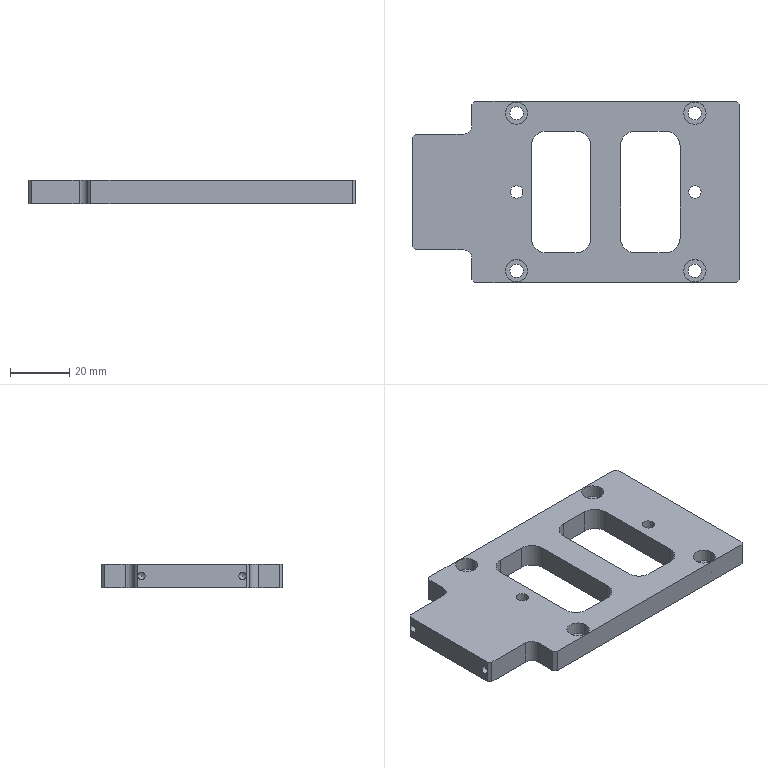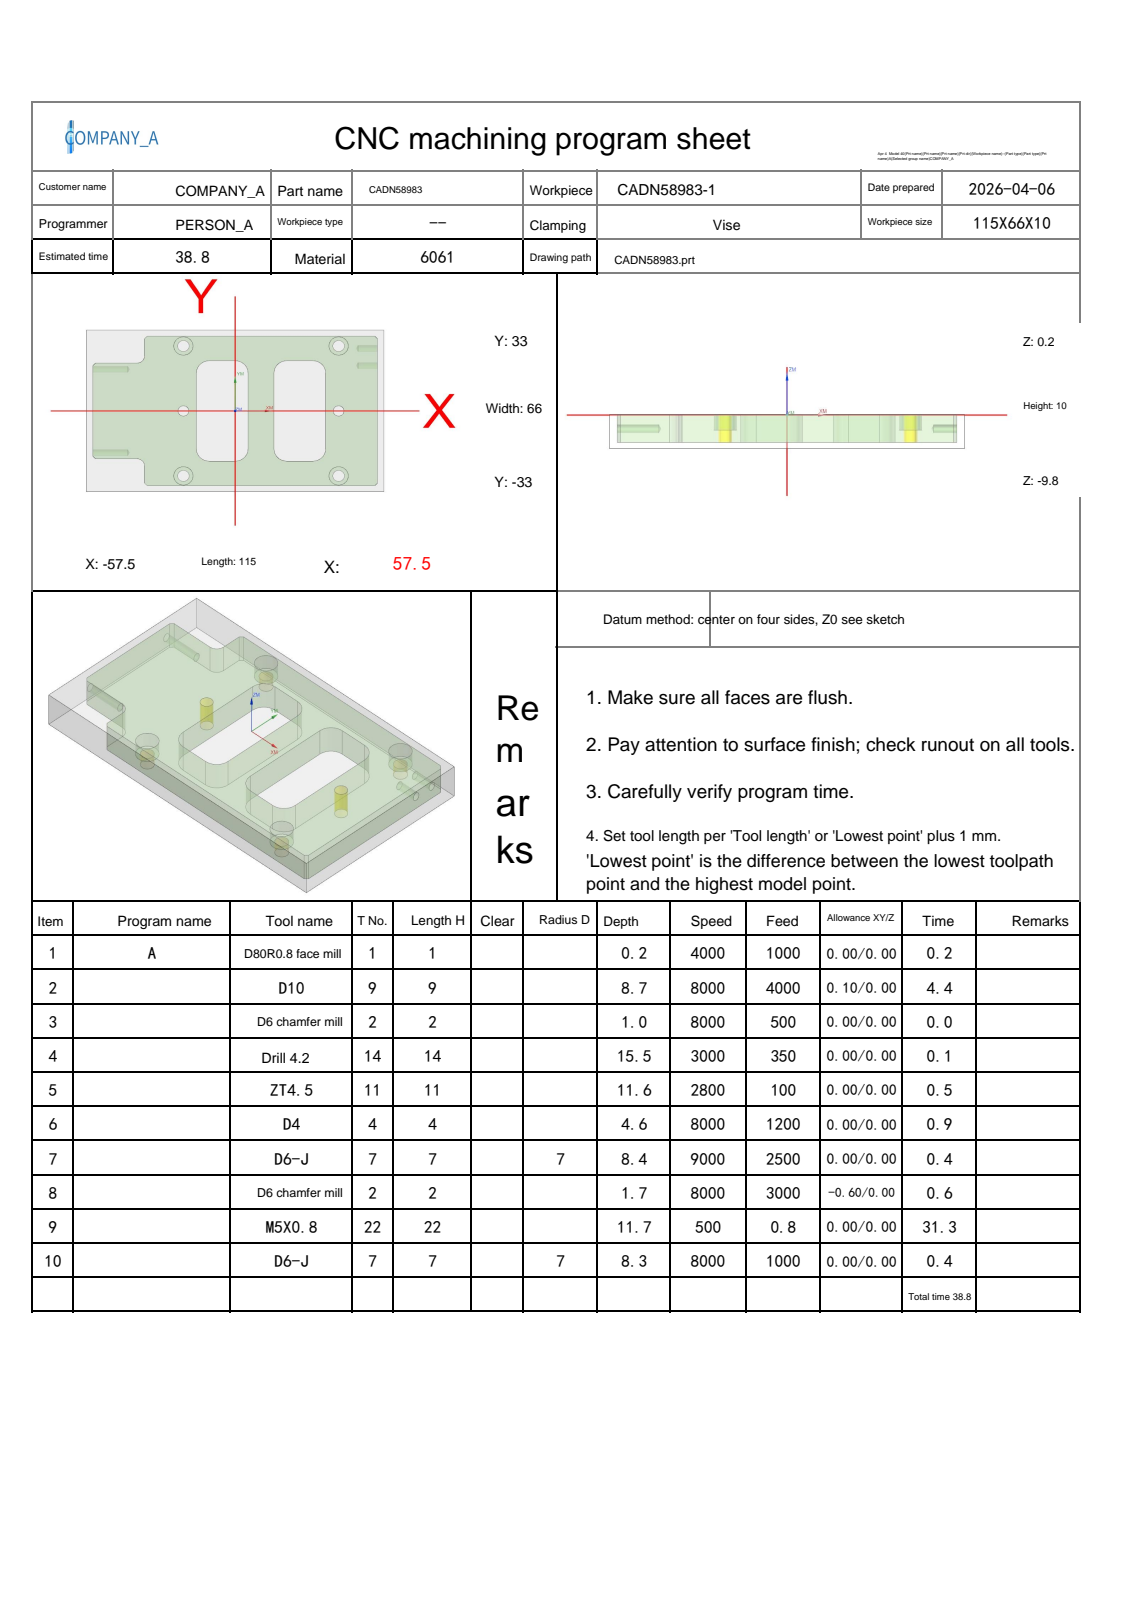NC program | NX | posted by the shop | part box 110 x 61 x 8 mm
Lines 4151 to 4510 of 4510:
N8 T02 M06
(D6 chamfer mill  D=6. R=0. H=02 ce=0.00 di=0.00)
G00 G90 G54 X9.75 Y32.628 M03 S8000
G43 H02 Z20.
M08
Z2.099
G01 Z-1.5 F3000.
G03 X9.67 Y32.328 I.52 J-.3
X9.97 Y31.808 I.6 J0.0
G01 X10. Y31.8
X54.
X54.254 Y31.775
X54.497 Y31.701
X54.722 Y31.581
X54.919 Y31.419
X55.919 Y30.419
X56.081 Y30.222
X56.201 Y29.997
X56.275 Y29.754
X56.3 Y29.5
Y-29.5
X56.275 Y-29.754
X56.201 Y-29.997
X56.081 Y-30.222
X55.919 Y-30.419
X54.919 Y-31.419
X54.722 Y-31.581
X54.497 Y-31.701
X54.254 Y-31.775
X54. Y-31.8
X-34.
X-34.254 Y-31.775
X-34.497 Y-31.701
X-34.722 Y-31.581
X-34.919 Y-31.419
X-35.919 Y-30.419
X-36.081 Y-30.222
X-36.201 Y-29.997
X-36.275 Y-29.754
X-36.3 Y-29.5
Y-22.5
G03 X-38. Y-20.8 I-1.7 J0.0
G01 X-54.
X-54.254 Y-20.775
X-54.497 Y-20.701
X-54.722 Y-20.581
X-54.919 Y-20.419
X-55.919 Y-19.419
X-56.081 Y-19.222
X-56.201 Y-18.997
X-56.275 Y-18.754
X-56.3 Y-18.5
Y18.5
X-56.275 Y18.754
X-56.201 Y18.997
X-56.081 Y19.222
X-55.919 Y19.419
X-54.919 Y20.419
X-54.722 Y20.581
X-54.497 Y20.701
X-54.254 Y20.775
X-54. Y20.8
X-38.
G03 X-36.3 Y22.5 I0.0 J1.7
G01 Y29.5
X-36.275 Y29.754
X-36.201 Y29.997
X-36.081 Y30.222
X-35.919 Y30.419
X-34.919 Y31.419
X-34.722 Y31.581
X-34.497 Y31.701
X-34.254 Y31.775
X-34. Y31.8
X10.
X10.03 Y31.808
G03 X10.33 Y32.328 I-.3 J.52
X10.25 Y32.628 I-.6 J0.0
G01 Z2.099
G00 Z20.
X2.872 Y-.25
Z2.099
G01 Z-1.5
G03 X3.172 Y-.33 I.3 J.52
X3.692 Y-.03 I0.0 J.6
G01 X3.7 Y0.0
Y15.5
G03 X0.0 Y19.2 I-3.7 J0.0
G01 X-10.
G03 X-13.7 Y15.5 I0.0 J-3.7
G01 Y-15.5
G03 X-10. Y-19.2 I3.7 J0.0
G01 X0.0
G03 X3.7 Y-15.5 I0.0 J3.7
G01 Y0.0
X3.692 Y.03
G03 X3.172 Y.33 I-.52 J-.3
X2.872 Y.25 I0.0 J-.6
G01 Z2.099
G00 Z20.
X17.128
Z2.099
G01 Z-1.5
G03 X16.828 Y.33 I-.3 J-.52
X16.308 Y.03 I0.0 J-.6
G01 X16.3 Y0.0
Y-15.5
G03 X20. Y-19.2 I3.7 J0.0
G01 X30.
G03 X33.7 Y-15.5 I0.0 J3.7
G01 Y15.5
G03 X30. Y19.2 I-3.7 J0.0
G01 X20.
G03 X16.3 Y15.5 I0.0 J-3.7
G01 Y0.0
X16.308 Y-.03
G03 X16.828 Y-.33 I.52 J.3
X17.128 Y-.25 I0.0 J.6
G01 Z2.099
G00 Z20.
G00 G90 X-19.907 Y-.694 M03 S8000
Z20.
Z-.5
G01 Z-1. F500.
X-19.8 Y-1.5
G03 X-18.3 Y0.0 I0.0 J1.5
X-20. Y1.7 I-1.7 J0.0
X-21.7 Y0.0 I0.0 J-1.7
X-20. Y-1.7 I1.7 J0.0
X-18.3 Y0.0 I0.0 J1.7
X-19.8 Y1.5 I-1.5 J0.0
G01 X-19.907 Y.694
Z-.5
G00 Z20.
X40.093 Y-.694
Z-.5
G01 Z-1.
X40.2 Y-1.5
G03 X41.7 Y0.0 I0.0 J1.5
X40. Y1.7 I-1.7 J0.0
X38.3 Y0.0 I0.0 J-1.7
X40. Y-1.7 I1.7 J0.0
X41.7 Y0.0 I0.0 J1.7
X40.2 Y1.5 I-1.5 J0.0
G01 X40.093 Y.694
Z-.5
G00 Z20.
G00 G90 X36.949 Y-26.469 M03 S8000
Z20.
Z2.5
G01 X36.947 Y-26.5 Z2.489 F500.
X36.971 Y-26.882 Z2.349
X37.042 Y-27.257 Z2.21
X37.16 Y-27.621 Z2.071
X37.323 Y-27.968 Z1.932
X37.527 Y-28.291 Z1.793
X37.771 Y-28.586 Z1.653
X38.049 Y-28.848 Z1.514
X38.358 Y-29.074 Z1.375
X38.592 Y-29.209 Z1.277
X38.942 Y-29.364 Z1.137
X39.308 Y-29.474 Z.998
X39.686 Y-29.537 Z.859
X40.068 Y-29.552 Z.72
X40.449 Y-29.52 Z.581
X40.823 Y-29.44 Z.441
X41.184 Y-29.314 Z.302
X41.527 Y-29.144 Z.163
X41.845 Y-28.932 Z.024
X42.135 Y-28.683 Z-.116
X42.391 Y-28.399 Z-.255
X42.609 Y-28.085 Z-.394
X42.787 Y-27.746 Z-.533
X42.921 Y-27.388 Z-.672
X43.009 Y-27.016 Z-.812
X43.05 Y-26.635 Z-.951
Y-26.5 Z-1.
G03 X40. Y-23.45 I-3.05 J0.0
X36.95 Y-26.5 I0.0 J-3.05
X40. Y-29.55 I3.05 J0.0
X43.05 Y-26.5 I0.0 J3.05
X43.009 Y-26.002 I-3.05 J0.0
G01 Z1.5
G00 Z20.
X36.949 Y26.531
Z2.5
G01 X36.947 Y26.5 Z2.489
X36.971 Y26.118 Z2.349
X37.042 Y25.743 Z2.21
X37.16 Y25.379 Z2.071
X37.323 Y25.032 Z1.932
X37.527 Y24.709 Z1.793
X37.771 Y24.414 Z1.653
X38.049 Y24.152 Z1.514
X38.358 Y23.926 Z1.375
X38.592 Y23.791 Z1.277
X38.942 Y23.636 Z1.137
X39.308 Y23.526 Z.998
X39.686 Y23.463 Z.859
X40.068 Y23.448 Z.72
X40.449 Y23.48 Z.581
X40.823 Y23.56 Z.441
X41.184 Y23.686 Z.302
X41.527 Y23.856 Z.163
X41.845 Y24.068 Z.024
X42.135 Y24.317 Z-.116
X42.391 Y24.601 Z-.255
X42.609 Y24.915 Z-.394
X42.787 Y25.254 Z-.533
X42.921 Y25.612 Z-.672
X43.009 Y25.984 Z-.812
X43.05 Y26.365 Z-.951
Y26.5 Z-1.
G03 X40. Y29.55 I-3.05 J0.0
X36.95 Y26.5 I0.0 J-3.05
X40. Y23.45 I3.05 J0.0
X43.05 Y26.5 I0.0 J3.05
X43.009 Y26.998 I-3.05 J0.0
G01 Z1.5
G00 Z20.
X-23.051 Y26.531
Z2.5
G01 X-23.053 Y26.5 Z2.489
X-23.029 Y26.118 Z2.349
X-22.958 Y25.743 Z2.21
X-22.84 Y25.379 Z2.071
X-22.677 Y25.032 Z1.932
X-22.473 Y24.709 Z1.793
X-22.229 Y24.414 Z1.653
X-21.951 Y24.152 Z1.514
X-21.642 Y23.926 Z1.375
X-21.408 Y23.791 Z1.277
X-21.058 Y23.636 Z1.137
X-20.692 Y23.526 Z.998
X-20.314 Y23.463 Z.859
X-19.932 Y23.448 Z.72
X-19.551 Y23.48 Z.581
X-19.177 Y23.56 Z.441
X-18.816 Y23.686 Z.302
X-18.474 Y23.856 Z.163
X-18.155 Y24.068 Z.024
X-17.865 Y24.317 Z-.116
X-17.609 Y24.601 Z-.255
X-17.391 Y24.915 Z-.394
X-17.213 Y25.254 Z-.533
X-17.079 Y25.612 Z-.672
X-16.991 Y25.984 Z-.812
X-16.95 Y26.365 Z-.951
Y26.5 Z-1.
G03 X-20. Y29.55 I-3.05 J0.0
X-23.05 Y26.5 I0.0 J-3.05
X-20. Y23.45 I3.05 J0.0
X-16.95 Y26.5 I0.0 J3.05
X-16.991 Y26.998 I-3.05 J0.0
G01 Z1.5
G00 Z20.
X-23.051 Y-26.469
Z2.5
G01 X-23.053 Y-26.5 Z2.489
X-23.029 Y-26.882 Z2.349
X-22.958 Y-27.257 Z2.21
X-22.84 Y-27.621 Z2.071
X-22.677 Y-27.968 Z1.932
X-22.473 Y-28.291 Z1.793
X-22.229 Y-28.586 Z1.653
X-21.951 Y-28.848 Z1.514
X-21.642 Y-29.074 Z1.375
X-21.408 Y-29.209 Z1.277
X-21.058 Y-29.364 Z1.137
X-20.692 Y-29.474 Z.998
X-20.314 Y-29.537 Z.859
X-19.932 Y-29.552 Z.72
X-19.551 Y-29.52 Z.581
X-19.177 Y-29.44 Z.441
X-18.816 Y-29.314 Z.302
X-18.474 Y-29.144 Z.163
X-18.155 Y-28.932 Z.024
X-17.865 Y-28.683 Z-.116
X-17.609 Y-28.399 Z-.255
X-17.391 Y-28.085 Z-.394
X-17.213 Y-27.746 Z-.533
X-17.079 Y-27.388 Z-.672
X-16.991 Y-27.016 Z-.812
X-16.95 Y-26.635 Z-.951
Y-26.5 Z-1.
G03 X-20. Y-23.45 I-3.05 J0.0
X-23.05 Y-26.5 I0.0 J-3.05
X-20. Y-29.55 I3.05 J0.0
X-16.95 Y-26.5 I0.0 J3.05
X-16.991 Y-26.002 I-3.05 J0.0
G01 Z1.5
G00 Z20.
G91 G28 Z0.0
M05
M09
G91 G28 Z0.0
M01
N9 T22 M06
(M5X0.8 D=4.2 DR_a=180 H=22)
G00 G90 G54 X-20. Y0.0 M03 S500
G43 H22 Z20.
M08
G95
G98 G84 X-20. Y0.0 Z-11.5 R1. F.8 Q3.
X40.
G80
G94
G00 Z20.
G91 G28 Z0.0
M05
M09
G91 G28 Z0.0
M01
N10 T07 M06
(D6-J  D=6. R=0. H=07 ce=0.00 di=0.00)
G00 G90 G54 X-35.017 Y34.573 M03 S8000
G43 H07 Z20.
M08
Z-7.6
G01 Z-8.1 F1000.
G41 D07
X-34.992 Y34.375
G03 X-34. Y33.5 I.992 J.125
G01 X54.
G02 X56.121 Y32.621 I0.0 J-3.
G01 X57.121 Y31.621
G02 X58. Y29.5 I-2.121 J-2.121
G01 Y-29.5
G02 X57.121 Y-31.621 I-3. J0.0
G01 X56.121 Y-32.621
G02 X54. Y-33.5 I-2.121 J2.121
G01 X-34.
G02 X-36.121 Y-32.621 I0.0 J3.
G01 X-37.121 Y-31.621
G02 X-38. Y-29.5 I2.121 J2.121
G01 Y-22.5
X-54.
G02 X-56.121 Y-21.621 I0.0 J3.
G01 X-57.121 Y-20.621
G02 X-58. Y-18.5 I2.121 J2.121
G01 Y18.5
G02 X-57.121 Y20.621 I3. J0.0
G01 X-56.121 Y21.621
G02 X-54. Y22.5 I2.121 J-2.121
G01 X-38.
Y29.5
G02 X-37.121 Y31.621 I3. J0.0
G01 X-36.121 Y32.621
G02 X-34. Y33.5 I2.121 J-2.121
G01 X-33.5
G03 X-32.5 Y34.5 I0.0 J1.
G01 G40 Y34.7
Z-7.6
G00 Z20.
M05
M09
G91 G28 Z0.0
G91 G28 Y0.0
M30
%